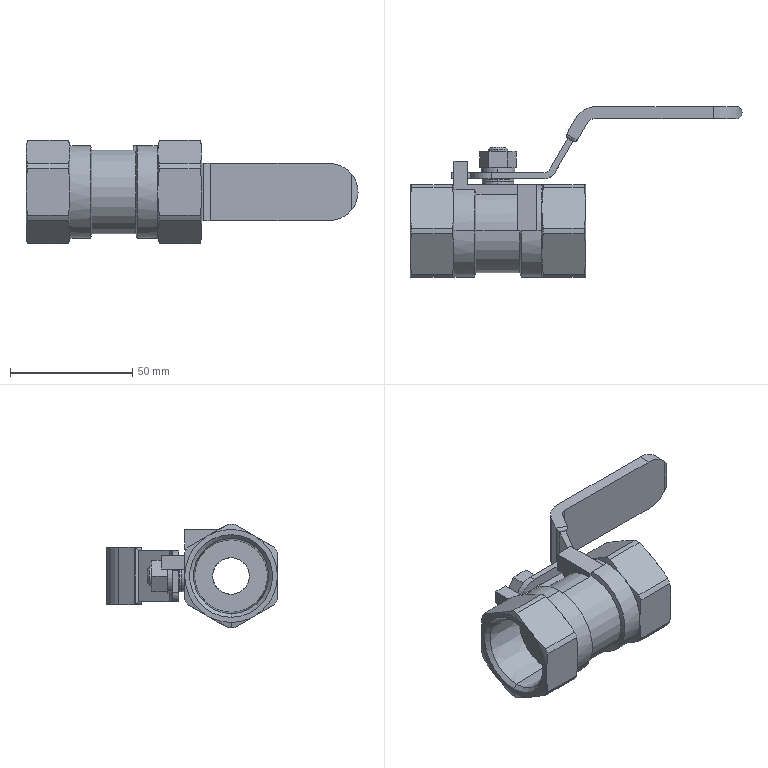Part | SolidWorks | features BaseBody 3 | 3 solids | 184 faces | box 136 x 70.001 x 42.56 mm | volume 63816 mm3 | cone 68 | cylinder 57 | plane 55 | sphere 4 | commonest cylinder face diameters 42.56 x14 15 x6 2.5 x5 38 x5 9 x4 13 x4